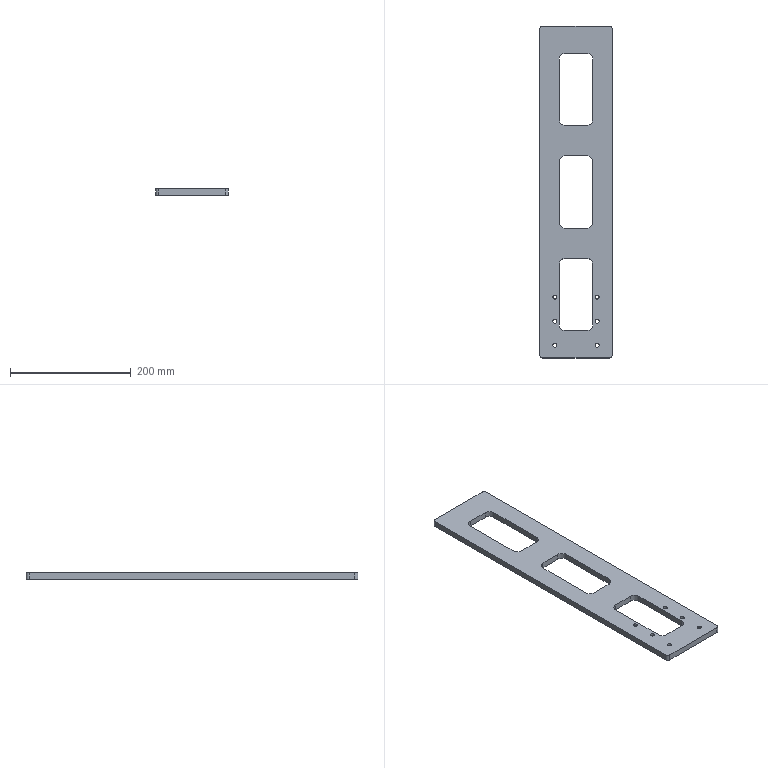Part | STEP file | PN_0011 | 1 solid | 64 faces | box 120 x 550 x 10 mm | volume 459826 mm3 | cylinder 40 | plane 24 | commonest cylinder face diameters 6.6 x12 11 x12 20 x12 10 x4